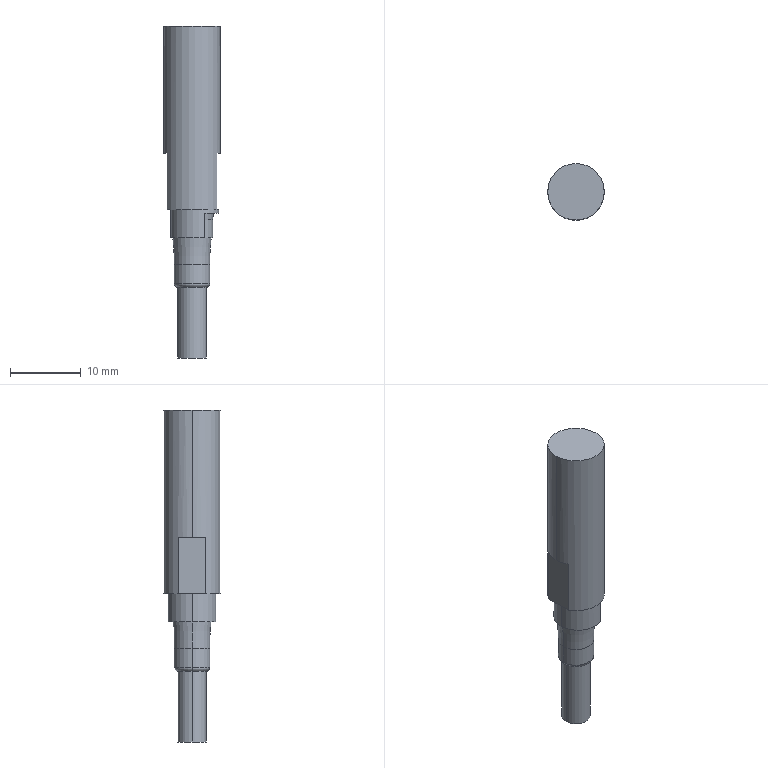Part | STEP file | E2E_X2D1_N_BASE | 1 solid | 27 faces | box 8 x 8 x 47 mm | volume 1680 mm3 | plane 12 | cylinder 9 | torus 4 | cone 2 | commonest cylinder face diameters 4 x2 5 x2 6.8 x2 8 x2 5.86 x1